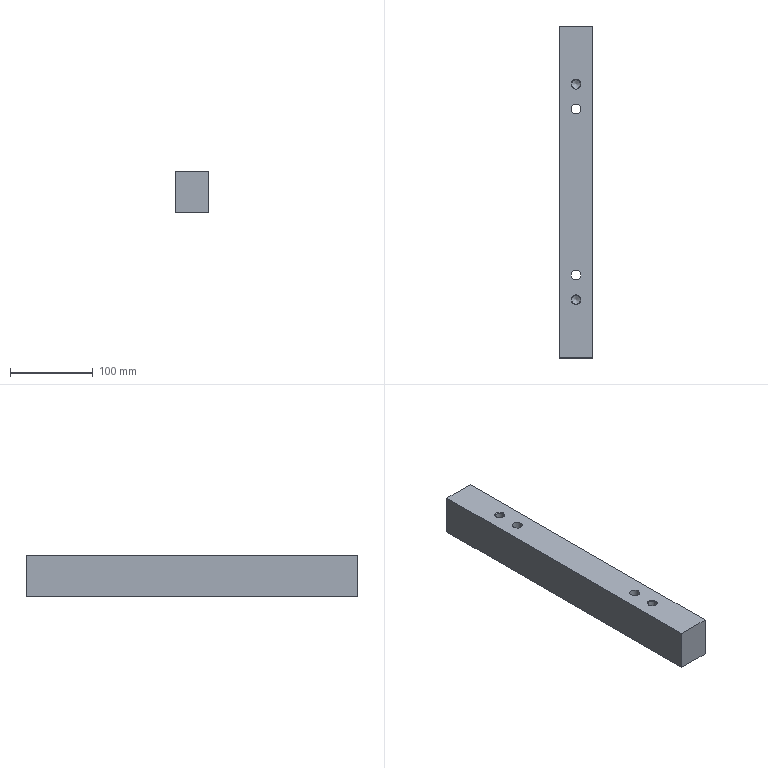Part | STEP file | gslz 2016.10.28-6_id958_x_t | 1 solid | 18 faces | box 40 x 400 x 50 mm | volume 781861 mm3 | plane 8 | cylinder 6 | cone 4 | commonest cylinder face diameters 10.3 x2 12 x2 14 x2
STEP:
#1=CARTESIAN_POINT('',(-225.,350.,-100.));
#2=VERTEX_POINT('',#1);
#3=CARTESIAN_POINT('',(-225.,350.,-50.));
#4=VERTEX_POINT('',#3);
#5=CARTESIAN_POINT('',(-225.,350.,-100.));
#6=DIRECTION('',(0.,0.,1.));
#7=VECTOR('',#6,1.);
#8=LINE('',#5,#7);
#9=EDGE_CURVE('',#2,#4,#8,.T.);
#10=ORIENTED_EDGE('',*,*,#9,.F.);
#11=CARTESIAN_POINT('',(-265.,350.,-100.));
#12=VERTEX_POINT('',#11);
#13=CARTESIAN_POINT('',(5.,350.,-100.));
#14=DIRECTION('',(-1.,0.,0.));
#15=VECTOR('',#14,1.);
#16=LINE('',#13,#15);
#17=EDGE_CURVE('',#2,#12,#16,.T.);
#18=ORIENTED_EDGE('',*,*,#17,.T.);
#19=CARTESIAN_POINT('',(-265.,350.,-50.));
#20=VERTEX_POINT('',#19);
#21=CARTESIAN_POINT('',(-265.,350.,-100.));
#22=DIRECTION('',(0.,0.,1.));
#23=VECTOR('',#22,1.);
#24=LINE('',#21,#23);
#25=EDGE_CURVE('',#12,#20,#24,.T.);
#26=ORIENTED_EDGE('',*,*,#25,.T.);
#27=CARTESIAN_POINT('',(5.,350.,-50.));
#28=DIRECTION('',(-1.,0.,0.));
#29=VECTOR('',#28,1.);
#30=LINE('',#27,#29);
#31=EDGE_CURVE('',#4,#20,#30,.T.);
#32=ORIENTED_EDGE('',*,*,#31,.F.);
#33=EDGE_LOOP('',(#10,#18,#26,#32));
#34=FACE_OUTER_BOUND('',#33,.T.);
#35=CARTESIAN_POINT('',(5.,350.,-100.));
#36=DIRECTION('',(0.,1.,0.));
#37=DIRECTION('',(0.,0.,-1.));
#38=AXIS2_PLACEMENT_3D('',#35,#36,#37);
#39=PLANE('',#38);
#40=ADVANCED_FACE('',(#34),#39,.T.);
#41=CARTESIAN_POINT('',(-225.,-50.,-50.));
#42=VERTEX_POINT('',#41);
#43=CARTESIAN_POINT('',(-225.,150.,-50.));
#44=DIRECTION('',(0.,-1.,0.));
#45=VECTOR('',#44,1.);
#46=LINE('',#43,#45);
#47=EDGE_CURVE('',#4,#42,#46,.T.);
#48=ORIENTED_EDGE('',*,*,#47,.T.);
#49=CARTESIAN_POINT('',(-225.,-50.,-100.));
#50=VERTEX_POINT('',#49);
#51=CARTESIAN_POINT('',(-225.,-50.,-100.));
#52=DIRECTION('',(0.,0.,-1.));
#53=VECTOR('',#52,1.);
#54=LINE('',#51,#53);
#55=EDGE_CURVE('',#42,#50,#54,.T.);
#56=ORIENTED_EDGE('',*,*,#55,.T.);
#57=CARTESIAN_POINT('',(-225.,150.,-100.));
#58=DIRECTION('',(0.,-1.,0.));
#59=VECTOR('',#58,1.);
#60=LINE('',#57,#59);
#61=EDGE_CURVE('',#2,#50,#60,.T.);
#62=ORIENTED_EDGE('',*,*,#61,.F.);
#63=ORIENTED_EDGE('',*,*,#9,.T.);
#64=EDGE_LOOP('',(#48,#56,#62,#63));
#65=FACE_OUTER_BOUND('',#64,.T.);
#66=CARTESIAN_POINT('',(-225.,150.,-221.492));
#67=DIRECTION('',(-1.,0.,0.));
#68=DIRECTION('',(0.,0.,-1.));
#69=AXIS2_PLACEMENT_3D('',#66,#67,#68);
#70=PLANE('',#69);
#71=ADVANCED_FACE('',(#65),#70,.F.);
#72=ORIENTED_EDGE('',*,*,#55,.F.);
#73=CARTESIAN_POINT('',(-265.,-50.,-50.));
#74=VERTEX_POINT('',#73);
#75=CARTESIAN_POINT('',(5.,-50.,-50.));
#76=DIRECTION('',(1.,0.,0.));
#77=VECTOR('',#76,1.);
#78=LINE('',#75,#77);
#79=EDGE_CURVE('',#74,#42,#78,.T.);
#80=ORIENTED_EDGE('',*,*,#79,.F.);
#81=CARTESIAN_POINT('',(-265.,-50.,-100.));
#82=VERTEX_POINT('',#81);
#83=CARTESIAN_POINT('',(-265.,-50.,-221.492));
#84=DIRECTION('',(0.,0.,1.));
#85=VECTOR('',#84,1.);
#86=LINE('',#83,#85);
#87=EDGE_CURVE('',#82,#74,#86,.T.);
#88=ORIENTED_EDGE('',*,*,#87,.F.);
#89=CARTESIAN_POINT('',(5.,-50.,-100.));
#90=DIRECTION('',(1.,0.,0.));
#91=VECTOR('',#90,1.);
#92=LINE('',#89,#91);
#93=EDGE_CURVE('',#82,#50,#92,.T.);
#94=ORIENTED_EDGE('',*,*,#93,.T.);
#95=EDGE_LOOP('',(#72,#80,#88,#94));
#96=FACE_OUTER_BOUND('',#95,.T.);
#97=CARTESIAN_POINT('',(5.,-50.,-100.));
#98=DIRECTION('',(0.,-1.,0.));
#99=DIRECTION('',(0.,0.,1.));
#100=AXIS2_PLACEMENT_3D('',#97,#98,#99);
#101=PLANE('',#100);
#102=ADVANCED_FACE('',(#96),#101,.T.);
#103=ORIENTED_EDGE('',*,*,#87,.T.);
#104=CARTESIAN_POINT('',(-265.,150.,-50.));
#105=DIRECTION('',(0.,-1.,0.));
#106=VECTOR('',#105,1.);
#107=LINE('',#104,#106);
#108=EDGE_CURVE('',#20,#74,#107,.T.);
#109=ORIENTED_EDGE('',*,*,#108,.F.);
#110=ORIENTED_EDGE('',*,*,#25,.F.);
#111=CARTESIAN_POINT('',(-265.,150.,-100.));
#112=DIRECTION('',(0.,-1.,0.));
#113=VECTOR('',#112,1.);
#114=LINE('',#111,#113);
#115=EDGE_CURVE('',#12,#82,#114,.T.);
#116=ORIENTED_EDGE('',*,*,#115,.T.);
#117=EDGE_LOOP('',(#103,#109,#110,#116));
#118=FACE_OUTER_BOUND('',#117,.T.);
#119=CARTESIAN_POINT('',(-265.,150.,-221.492));
#120=DIRECTION('',(-1.,0.,0.));
#121=DIRECTION('',(0.,0.,-1.));
#122=AXIS2_PLACEMENT_3D('',#119,#120,#121);
#123=PLANE('',#122);
#124=ADVANCED_FACE('',(#118),#123,.T.);
#125=CARTESIAN_POINT('',(-251.,250.,-50.));
#126=VERTEX_POINT('',#125);
#127=CARTESIAN_POINT('',(-245.,250.,-50.));
#128=DIRECTION('',(0.,0.,-1.));
#129=DIRECTION('',(-1.,0.,0.));
#130=AXIS2_PLACEMENT_3D('',#127,#128,#129);
#131=CIRCLE('',#130,6.);
#132=EDGE_CURVE('',#126,#126,#131,.T.);
#133=ORIENTED_EDGE('',*,*,#132,.T.);
#134=EDGE_LOOP('',(#133));
#135=FACE_BOUND('',#134,.T.);
#136=CARTESIAN_POINT('',(-251.,50.,-50.));
#137=VERTEX_POINT('',#136);
#138=CARTESIAN_POINT('',(-245.,50.,-50.));
#139=DIRECTION('',(0.,0.,-1.));
#140=DIRECTION('',(-1.,0.,0.));
#141=AXIS2_PLACEMENT_3D('',#138,#139,#140);
#142=CIRCLE('',#141,6.);
#143=EDGE_CURVE('',#137,#137,#142,.T.);
#144=ORIENTED_EDGE('',*,*,#143,.T.);
#145=EDGE_LOOP('',(#144));
#146=FACE_BOUND('',#145,.T.);
#147=ORIENTED_EDGE('',*,*,#79,.T.);
#148=ORIENTED_EDGE('',*,*,#47,.F.);
#149=ORIENTED_EDGE('',*,*,#31,.T.);
#150=ORIENTED_EDGE('',*,*,#108,.T.);
#151=EDGE_LOOP('',(#147,#148,#149,#150));
#152=FACE_BOUND('',#151,.T.);
#153=CARTESIAN_POINT('',(-251.,20.,-50.));
#154=VERTEX_POINT('',#153);
#155=CARTESIAN_POINT('',(-245.,20.,-50.));
#156=DIRECTION('',(0.,0.,1.));
#157=DIRECTION('',(-1.,0.,0.));
#158=AXIS2_PLACEMENT_3D('',#155,#156,#157);
#159=CIRCLE('',#158,6.);
#160=EDGE_CURVE('',#154,#154,#159,.T.);
#161=ORIENTED_EDGE('',*,*,#160,.F.);
#162=EDGE_LOOP('',(#161));
#163=FACE_BOUND('',#162,.T.);
#164=CARTESIAN_POINT('',(-251.,280.,-50.));
#165=VERTEX_POINT('',#164);
#166=CARTESIAN_POINT('',(-245.,280.,-50.));
#167=DIRECTION('',(0.,0.,1.));
#168=DIRECTION('',(-1.,0.,0.));
#169=AXIS2_PLACEMENT_3D('',#166,#167,#168);
#170=CIRCLE('',#169,6.);
#171=EDGE_CURVE('',#165,#165,#170,.T.);
#172=ORIENTED_EDGE('',*,*,#171,.F.);
#173=EDGE_LOOP('',(#172));
#174=FACE_BOUND('',#173,.T.);
#175=CARTESIAN_POINT('',(-5.,150.,-50.));
#176=DIRECTION('',(0.,0.,-1.));
#177=DIRECTION('',(1.,0.,0.));
#178=AXIS2_PLACEMENT_3D('',#175,#176,#177);
#179=PLANE('',#178);
#180=ADVANCED_FACE('',(#135,#146,#152,#163,#174),#179,.F.);
#181=CARTESIAN_POINT('',(-252.,250.,-100.));
#182=VERTEX_POINT('',#181);
#183=CARTESIAN_POINT('',(-245.,250.,-100.));
#184=DIRECTION('',(0.,0.,-1.));
#185=DIRECTION('',(-1.,0.,0.));
#186=AXIS2_PLACEMENT_3D('',#183,#184,#185);
#187=CIRCLE('',#186,7.);
#188=EDGE_CURVE('',#182,#182,#187,.T.);
#189=ORIENTED_EDGE('',*,*,#188,.F.);
#190=EDGE_LOOP('',(#189));
#191=FACE_BOUND('',#190,.T.);
#192=CARTESIAN_POINT('',(-252.,50.,-100.));
#193=VERTEX_POINT('',#192);
#194=CARTESIAN_POINT('',(-245.,50.,-100.));
#195=DIRECTION('',(0.,0.,-1.));
#196=DIRECTION('',(-1.,0.,0.));
#197=AXIS2_PLACEMENT_3D('',#194,#195,#196);
#198=CIRCLE('',#197,7.);
#199=EDGE_CURVE('',#193,#193,#198,.T.);
#200=ORIENTED_EDGE('',*,*,#199,.F.);
#201=EDGE_LOOP('',(#200));
#202=FACE_BOUND('',#201,.T.);
#203=ORIENTED_EDGE('',*,*,#61,.T.);
#204=ORIENTED_EDGE('',*,*,#93,.F.);
#205=ORIENTED_EDGE('',*,*,#115,.F.);
#206=ORIENTED_EDGE('',*,*,#17,.F.);
#207=EDGE_LOOP('',(#203,#204,#205,#206));
#208=FACE_BOUND('',#207,.T.);
#209=CARTESIAN_POINT('',(-5.,150.,-100.));
#210=DIRECTION('',(0.,0.,-1.));
#211=DIRECTION('',(1.,0.,0.));
#212=AXIS2_PLACEMENT_3D('',#209,#210,#211);
#213=PLANE('',#212);
#214=ADVANCED_FACE('',(#191,#202,#208),#213,.T.);
#215=CARTESIAN_POINT('',(-251.,50.,-80.));
#216=VERTEX_POINT('',#215);
#217=CARTESIAN_POINT('',(-245.,50.,-80.));
#218=DIRECTION('',(0.,0.,-1.));
#219=DIRECTION('',(-1.,0.,0.));
#220=AXIS2_PLACEMENT_3D('',#217,#218,#219);
#221=CIRCLE('',#220,6.);
#222=EDGE_CURVE('',#216,#216,#221,.T.);
#223=ORIENTED_EDGE('',*,*,#222,.T.);
#224=EDGE_LOOP('',(#223));
#225=FACE_BOUND('',#224,.T.);
#226=ORIENTED_EDGE('',*,*,#143,.F.);
#227=EDGE_LOOP('',(#226));
#228=FACE_BOUND('',#227,.T.);
#229=CARTESIAN_POINT('',(-245.,50.,-65.));
#230=DIRECTION('',(0.,0.,1.));
#231=DIRECTION('',(1.,0.,0.));
#232=AXIS2_PLACEMENT_3D('',#229,#230,#231);
#233=CYLINDRICAL_SURFACE('',#232,6.);
#234=ADVANCED_FACE('',(#225,#228),#233,.F.);
#235=CARTESIAN_POINT('',(-238.,50.,-80.));
#236=VERTEX_POINT('',#235);
#237=CARTESIAN_POINT('',(-245.,50.,-80.));
#238=DIRECTION('',(0.,0.,-1.));
#239=DIRECTION('',(1.,0.,0.));
#240=AXIS2_PLACEMENT_3D('',#237,#238,#239);
#241=CIRCLE('',#240,7.);
#242=EDGE_CURVE('',#236,#236,#241,.T.);
#243=ORIENTED_EDGE('',*,*,#242,.T.);
#244=EDGE_LOOP('',(#243));
#245=FACE_BOUND('',#244,.T.);
#246=ORIENTED_EDGE('',*,*,#222,.F.);
#247=EDGE_LOOP('',(#246));
#248=FACE_BOUND('',#247,.T.);
#249=CARTESIAN_POINT('',(-245.,50.,-80.));
#250=DIRECTION('',(0.,0.,1.));
#251=DIRECTION('',(-1.,0.,0.));
#252=AXIS2_PLACEMENT_3D('',#249,#250,#251);
#253=PLANE('',#252);
#254=ADVANCED_FACE('',(#245,#248),#253,.F.);
#255=ORIENTED_EDGE('',*,*,#199,.T.);
#256=EDGE_LOOP('',(#255));
#257=FACE_BOUND('',#256,.T.);
#258=ORIENTED_EDGE('',*,*,#242,.F.);
#259=EDGE_LOOP('',(#258));
#260=FACE_BOUND('',#259,.T.);
#261=CARTESIAN_POINT('',(-245.,50.,-85.));
#262=DIRECTION('',(0.,0.,1.));
#263=DIRECTION('',(1.,0.,0.));
#264=AXIS2_PLACEMENT_3D('',#261,#262,#263);
#265=CYLINDRICAL_SURFACE('',#264,7.);
#266=ADVANCED_FACE('',(#257,#260),#265,.F.);
#267=CARTESIAN_POINT('',(-250.15,20.,-80.));
#268=VERTEX_POINT('',#267);
#269=CARTESIAN_POINT('',(-245.,20.,-80.));
#270=DIRECTION('',(0.,0.,1.));
#271=DIRECTION('',(-1.,0.,0.));
#272=AXIS2_PLACEMENT_3D('',#269,#270,#271);
#273=CIRCLE('',#272,5.15);
#274=EDGE_CURVE('',#268,#268,#273,.T.);
#275=ORIENTED_EDGE('',*,*,#274,.T.);
#276=EDGE_LOOP('',(#275));
#277=FACE_BOUND('',#276,.T.);
#278=CARTESIAN_POINT('',(-245.,20.,-83.094));
#279=VERTEX_POINT('',#278);
#280=VERTEX_LOOP('',#279);
#281=FACE_BOUND('',#280,.T.);
#282=CARTESIAN_POINT('',(-245.,20.,-80.));
#283=DIRECTION('',(0.,0.,1.));
#284=DIRECTION('',(1.,0.,0.));
#285=AXIS2_PLACEMENT_3D('',#282,#283,#284);
#286=CONICAL_SURFACE('',#285,5.15,59.);
#287=ADVANCED_FACE('',(#277,#281),#286,.F.);
#288=CARTESIAN_POINT('',(-239.85,20.,-50.85));
#289=VERTEX_POINT('',#288);
#290=CARTESIAN_POINT('',(-245.,20.,-50.85));
#291=DIRECTION('',(0.,0.,-1.));
#292=DIRECTION('',(1.,0.,0.));
#293=AXIS2_PLACEMENT_3D('',#290,#291,#292);
#294=CIRCLE('',#293,5.15);
#295=EDGE_CURVE('',#289,#289,#294,.T.);
#296=ORIENTED_EDGE('',*,*,#295,.F.);
#297=EDGE_LOOP('',(#296));
#298=FACE_BOUND('',#297,.T.);
#299=ORIENTED_EDGE('',*,*,#274,.F.);
#300=EDGE_LOOP('',(#299));
#301=FACE_BOUND('',#300,.T.);
#302=CARTESIAN_POINT('',(-245.,20.,-50.));
#303=DIRECTION('',(0.,0.,-1.));
#304=DIRECTION('',(-1.,0.,0.));
#305=AXIS2_PLACEMENT_3D('',#302,#303,#304);
#306=CYLINDRICAL_SURFACE('',#305,5.15);
#307=ADVANCED_FACE('',(#298,#301),#306,.F.);
#308=ORIENTED_EDGE('',*,*,#295,.T.);
#309=EDGE_LOOP('',(#308));
#310=FACE_BOUND('',#309,.T.);
#311=ORIENTED_EDGE('',*,*,#160,.T.);
#312=EDGE_LOOP('',(#311));
#313=FACE_BOUND('',#312,.T.);
#314=CARTESIAN_POINT('',(-245.,20.,-50.));
#315=DIRECTION('',(0.,0.,1.));
#316=DIRECTION('',(-1.,0.,0.));
#317=AXIS2_PLACEMENT_3D('',#314,#315,#316);
#318=CONICAL_SURFACE('',#317,6.,45.);
#319=ADVANCED_FACE('',(#310,#313),#318,.F.);
#320=CARTESIAN_POINT('',(-250.15,280.,-80.));
#321=VERTEX_POINT('',#320);
#322=CARTESIAN_POINT('',(-245.,280.,-80.));
#323=DIRECTION('',(0.,0.,1.));
#324=DIRECTION('',(-1.,0.,0.));
#325=AXIS2_PLACEMENT_3D('',#322,#323,#324);
#326=CIRCLE('',#325,5.15);
#327=EDGE_CURVE('',#321,#321,#326,.T.);
#328=ORIENTED_EDGE('',*,*,#327,.T.);
#329=EDGE_LOOP('',(#328));
#330=FACE_BOUND('',#329,.T.);
#331=CARTESIAN_POINT('',(-245.,280.,-83.094));
#332=VERTEX_POINT('',#331);
#333=VERTEX_LOOP('',#332);
#334=FACE_BOUND('',#333,.T.);
#335=CARTESIAN_POINT('',(-245.,280.,-80.));
#336=DIRECTION('',(0.,0.,1.));
#337=DIRECTION('',(1.,0.,0.));
#338=AXIS2_PLACEMENT_3D('',#335,#336,#337);
#339=CONICAL_SURFACE('',#338,5.15,59.);
#340=ADVANCED_FACE('',(#330,#334),#339,.F.);
#341=CARTESIAN_POINT('',(-239.85,280.,-50.85));
#342=VERTEX_POINT('',#341);
#343=CARTESIAN_POINT('',(-245.,280.,-50.85));
#344=DIRECTION('',(0.,0.,-1.));
#345=DIRECTION('',(1.,0.,0.));
#346=AXIS2_PLACEMENT_3D('',#343,#344,#345);
#347=CIRCLE('',#346,5.15);
#348=EDGE_CURVE('',#342,#342,#347,.T.);
#349=ORIENTED_EDGE('',*,*,#348,.F.);
#350=EDGE_LOOP('',(#349));
#351=FACE_BOUND('',#350,.T.);
#352=ORIENTED_EDGE('',*,*,#327,.F.);
#353=EDGE_LOOP('',(#352));
#354=FACE_BOUND('',#353,.T.);
#355=CARTESIAN_POINT('',(-245.,280.,-50.));
#356=DIRECTION('',(0.,0.,-1.));
#357=DIRECTION('',(-1.,0.,0.));
#358=AXIS2_PLACEMENT_3D('',#355,#356,#357);
#359=CYLINDRICAL_SURFACE('',#358,5.15);
#360=ADVANCED_FACE('',(#351,#354),#359,.F.);
#361=ORIENTED_EDGE('',*,*,#348,.T.);
#362=EDGE_LOOP('',(#361));
#363=FACE_BOUND('',#362,.T.);
#364=ORIENTED_EDGE('',*,*,#171,.T.);
#365=EDGE_LOOP('',(#364));
#366=FACE_BOUND('',#365,.T.);
#367=CARTESIAN_POINT('',(-245.,280.,-50.));
#368=DIRECTION('',(0.,0.,1.));
#369=DIRECTION('',(-1.,0.,0.));
#370=AXIS2_PLACEMENT_3D('',#367,#368,#369);
#371=CONICAL_SURFACE('',#370,6.,45.);
#372=ADVANCED_FACE('',(#363,#366),#371,.F.);
#373=CARTESIAN_POINT('',(-251.,250.,-80.));
#374=VERTEX_POINT('',#373);
#375=CARTESIAN_POINT('',(-245.,250.,-80.));
#376=DIRECTION('',(0.,0.,-1.));
#377=DIRECTION('',(-1.,0.,0.));
#378=AXIS2_PLACEMENT_3D('',#375,#376,#377);
#379=CIRCLE('',#378,6.);
#380=EDGE_CURVE('',#374,#374,#379,.T.);
#381=ORIENTED_EDGE('',*,*,#380,.T.);
#382=EDGE_LOOP('',(#381));
#383=FACE_BOUND('',#382,.T.);
#384=ORIENTED_EDGE('',*,*,#132,.F.);
#385=EDGE_LOOP('',(#384));
#386=FACE_BOUND('',#385,.T.);
#387=CARTESIAN_POINT('',(-245.,250.,-65.));
#388=DIRECTION('',(0.,0.,1.));
#389=DIRECTION('',(-1.,0.,0.));
#390=AXIS2_PLACEMENT_3D('',#387,#388,#389);
#391=CYLINDRICAL_SURFACE('',#390,6.);
#392=ADVANCED_FACE('',(#383,#386),#391,.F.);
#393=CARTESIAN_POINT('',(-238.,250.,-80.));
#394=VERTEX_POINT('',#393);
#395=CARTESIAN_POINT('',(-245.,250.,-80.));
#396=DIRECTION('',(0.,0.,-1.));
#397=DIRECTION('',(1.,0.,0.));
#398=AXIS2_PLACEMENT_3D('',#395,#396,#397);
#399=CIRCLE('',#398,7.);
#400=EDGE_CURVE('',#394,#394,#399,.T.);
#401=ORIENTED_EDGE('',*,*,#400,.T.);
#402=EDGE_LOOP('',(#401));
#403=FACE_BOUND('',#402,.T.);
#404=ORIENTED_EDGE('',*,*,#380,.F.);
#405=EDGE_LOOP('',(#404));
#406=FACE_BOUND('',#405,.T.);
#407=CARTESIAN_POINT('',(-245.,250.,-80.));
#408=DIRECTION('',(0.,0.,1.));
#409=DIRECTION('',(-1.,0.,0.));
#410=AXIS2_PLACEMENT_3D('',#407,#408,#409);
#411=PLANE('',#410);
#412=ADVANCED_FACE('',(#403,#406),#411,.F.);
#413=ORIENTED_EDGE('',*,*,#188,.T.);
#414=EDGE_LOOP('',(#413));
#415=FACE_BOUND('',#414,.T.);
#416=ORIENTED_EDGE('',*,*,#400,.F.);
#417=EDGE_LOOP('',(#416));
#418=FACE_BOUND('',#417,.T.);
#419=CARTESIAN_POINT('',(-245.,250.,-85.));
#420=DIRECTION('',(0.,0.,1.));
#421=DIRECTION('',(1.,0.,0.));
#422=AXIS2_PLACEMENT_3D('',#419,#420,#421);
#423=CYLINDRICAL_SURFACE('',#422,7.);
#424=ADVANCED_FACE('',(#415,#418),#423,.F.);
#425=CLOSED_SHELL('',(#40,#71,#102,#124,#180,#214,#234,#254,#266,#287,#307,#319,#340,#360,#372,#392,#412,#424));
#426=MANIFOLD_SOLID_BREP('',#425);
#427=(LENGTH_UNIT()NAMED_UNIT(*)SI_UNIT(.MILLI.,.METRE.));
#428=UNCERTAINTY_MEASURE_WITH_UNIT(LENGTH_MEASURE(0.00002),#427,'','');
#429=(NAMED_UNIT(*)PLANE_ANGLE_UNIT()SI_UNIT($,.RADIAN.));
#430=PLANE_ANGLE_MEASURE_WITH_UNIT(PLANE_ANGLE_MEASURE(0.01745),#429);
#431=DIMENSIONAL_EXPONENTS(0.,0.,0.,0.,0.,0.,0.);
#432=(CONVERSION_BASED_UNIT('DEGREE',#430)NAMED_UNIT(#431)PLANE_ANGLE_UNIT());
#433=(NAMED_UNIT(*)SI_UNIT($,.STERADIAN.)SOLID_ANGLE_UNIT());
#434=(GEOMETRIC_REPRESENTATION_CONTEXT(3)GLOBAL_UNCERTAINTY_ASSIGNED_CONTEXT((#428))GLOBAL_UNIT_ASSIGNED_CONTEXT((#427,#432,#433))REPRESENTATION_CONTEXT('',''));
#435=ADVANCED_BREP_SHAPE_REPRESENTATION('',(#426),#434);